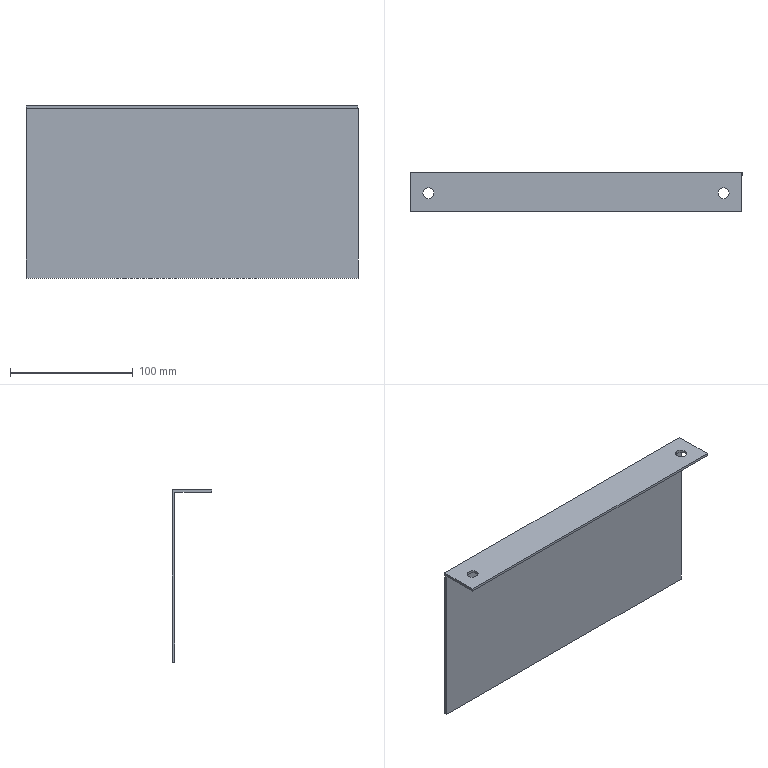Part | STEP file | lll_id2182_x_t | 1 solid | 10 faces | box 270 x 32 x 140 mm | volume 91546 mm3 | plane 8 | cylinder 2 | commonest cylinder face diameters 9 x2
STEP:
#1=CARTESIAN_POINT('',(554.935,-441.,2.5));
#2=VERTEX_POINT('',#1);
#3=CARTESIAN_POINT('',(554.935,-439.,2.5));
#4=VERTEX_POINT('',#3);
#5=CARTESIAN_POINT('',(554.935,-441.,2.5));
#6=DIRECTION('',(0.,1.,0.));
#7=VECTOR('',#6,1.);
#8=LINE('',#5,#7);
#9=EDGE_CURVE('',#2,#4,#8,.T.);
#10=ORIENTED_EDGE('',*,*,#9,.T.);
#11=CARTESIAN_POINT('',(824.935,-439.,2.5));
#12=VERTEX_POINT('',#11);
#13=CARTESIAN_POINT('',(499.935,-439.,2.5));
#14=DIRECTION('',(1.,0.,0.));
#15=VECTOR('',#14,1.);
#16=LINE('',#13,#15);
#17=EDGE_CURVE('',#4,#12,#16,.T.);
#18=ORIENTED_EDGE('',*,*,#17,.T.);
#19=CARTESIAN_POINT('',(824.935,-441.,2.5));
#20=VERTEX_POINT('',#19);
#21=CARTESIAN_POINT('',(824.935,45.,2.5));
#22=DIRECTION('',(0.,1.,0.));
#23=VECTOR('',#22,1.);
#24=LINE('',#21,#23);
#25=EDGE_CURVE('',#20,#12,#24,.T.);
#26=ORIENTED_EDGE('',*,*,#25,.F.);
#27=CARTESIAN_POINT('',(499.935,-441.,2.5));
#28=DIRECTION('',(1.,0.,0.));
#29=VECTOR('',#28,1.);
#30=LINE('',#27,#29);
#31=EDGE_CURVE('',#2,#20,#30,.T.);
#32=ORIENTED_EDGE('',*,*,#31,.F.);
#33=EDGE_LOOP('',(#10,#18,#26,#32));
#34=FACE_OUTER_BOUND('',#33,.T.);
#35=CARTESIAN_POINT('',(1692.435,45.,2.5));
#36=DIRECTION('',(0.,0.,-1.));
#37=DIRECTION('',(-1.,0.,0.));
#38=AXIS2_PLACEMENT_3D('',#35,#36,#37);
#39=PLANE('',#38);
#40=ADVANCED_FACE('',(#34),#39,.T.);
#41=CARTESIAN_POINT('',(824.935,-441.,140.5));
#42=VERTEX_POINT('',#41);
#43=CARTESIAN_POINT('',(554.935,-441.,140.5));
#44=VERTEX_POINT('',#43);
#45=CARTESIAN_POINT('',(499.935,-441.,140.5));
#46=DIRECTION('',(-1.,0.,0.));
#47=VECTOR('',#46,1.);
#48=LINE('',#45,#47);
#49=EDGE_CURVE('',#42,#44,#48,.T.);
#50=ORIENTED_EDGE('',*,*,#49,.T.);
#51=CARTESIAN_POINT('',(554.935,-441.,142.5));
#52=DIRECTION('',(0.,0.,-1.));
#53=VECTOR('',#52,1.);
#54=LINE('',#51,#53);
#55=EDGE_CURVE('',#44,#2,#54,.T.);
#56=ORIENTED_EDGE('',*,*,#55,.T.);
#57=ORIENTED_EDGE('',*,*,#31,.T.);
#58=CARTESIAN_POINT('',(824.935,-441.,-78.5));
#59=DIRECTION('',(0.,0.,1.));
#60=VECTOR('',#59,1.);
#61=LINE('',#58,#60);
#62=EDGE_CURVE('',#20,#42,#61,.T.);
#63=ORIENTED_EDGE('',*,*,#62,.T.);
#64=EDGE_LOOP('',(#50,#56,#57,#63));
#65=FACE_OUTER_BOUND('',#64,.T.);
#66=CARTESIAN_POINT('',(499.935,-441.,-78.5));
#67=DIRECTION('',(0.,1.,0.));
#68=DIRECTION('',(0.,0.,-1.));
#69=AXIS2_PLACEMENT_3D('',#66,#67,#68);
#70=PLANE('',#69);
#71=ADVANCED_FACE('',(#65),#70,.F.);
#72=CARTESIAN_POINT('',(554.935,-439.,142.5));
#73=VERTEX_POINT('',#72);
#74=CARTESIAN_POINT('',(554.935,-439.,-78.5));
#75=DIRECTION('',(0.,0.,-1.));
#76=VECTOR('',#75,1.);
#77=LINE('',#74,#76);
#78=EDGE_CURVE('',#73,#4,#77,.T.);
#79=ORIENTED_EDGE('',*,*,#78,.F.);
#80=CARTESIAN_POINT('',(824.935,-439.,142.5));
#81=VERTEX_POINT('',#80);
#82=CARTESIAN_POINT('',(499.935,-439.,142.5));
#83=DIRECTION('',(-1.,0.,0.));
#84=VECTOR('',#83,1.);
#85=LINE('',#82,#84);
#86=EDGE_CURVE('',#81,#73,#85,.T.);
#87=ORIENTED_EDGE('',*,*,#86,.F.);
#88=CARTESIAN_POINT('',(824.935,-439.,-78.5));
#89=DIRECTION('',(0.,0.,1.));
#90=VECTOR('',#89,1.);
#91=LINE('',#88,#90);
#92=EDGE_CURVE('',#12,#81,#91,.T.);
#93=ORIENTED_EDGE('',*,*,#92,.F.);
#94=ORIENTED_EDGE('',*,*,#17,.F.);
#95=EDGE_LOOP('',(#79,#87,#93,#94));
#96=FACE_OUTER_BOUND('',#95,.T.);
#97=CARTESIAN_POINT('',(499.935,-439.,-78.5));
#98=DIRECTION('',(0.,1.,0.));
#99=DIRECTION('',(0.,0.,-1.));
#100=AXIS2_PLACEMENT_3D('',#97,#98,#99);
#101=PLANE('',#100);
#102=ADVANCED_FACE('',(#96),#101,.T.);
#103=ORIENTED_EDGE('',*,*,#9,.F.);
#104=ORIENTED_EDGE('',*,*,#55,.F.);
#105=CARTESIAN_POINT('',(554.935,-471.,140.5));
#106=VERTEX_POINT('',#105);
#107=CARTESIAN_POINT('',(554.935,-441.,140.5));
#108=DIRECTION('',(0.,1.,0.));
#109=VECTOR('',#108,1.);
#110=LINE('',#107,#109);
#111=EDGE_CURVE('',#106,#44,#110,.T.);
#112=ORIENTED_EDGE('',*,*,#111,.F.);
#113=CARTESIAN_POINT('',(554.935,-471.,142.5));
#114=VERTEX_POINT('',#113);
#115=CARTESIAN_POINT('',(554.935,-471.,142.5));
#116=DIRECTION('',(0.,0.,-1.));
#117=VECTOR('',#116,1.);
#118=LINE('',#115,#117);
#119=EDGE_CURVE('',#114,#106,#118,.T.);
#120=ORIENTED_EDGE('',*,*,#119,.F.);
#121=CARTESIAN_POINT('',(554.935,-441.,142.5));
#122=DIRECTION('',(0.,1.,0.));
#123=VECTOR('',#122,1.);
#124=LINE('',#121,#123);
#125=EDGE_CURVE('',#114,#73,#124,.T.);
#126=ORIENTED_EDGE('',*,*,#125,.T.);
#127=ORIENTED_EDGE('',*,*,#78,.T.);
#128=EDGE_LOOP('',(#103,#104,#112,#120,#126,#127));
#129=FACE_OUTER_BOUND('',#128,.T.);
#130=CARTESIAN_POINT('',(554.935,-441.,142.5));
#131=DIRECTION('',(-1.,0.,0.));
#132=DIRECTION('',(0.,0.,-1.));
#133=AXIS2_PLACEMENT_3D('',#130,#131,#132);
#134=PLANE('',#133);
#135=ADVANCED_FACE('',(#129),#134,.T.);
#136=ORIENTED_EDGE('',*,*,#119,.T.);
#137=CARTESIAN_POINT('',(824.935,-471.,140.5));
#138=VERTEX_POINT('',#137);
#139=CARTESIAN_POINT('',(499.935,-471.,140.5));
#140=DIRECTION('',(-1.,0.,0.));
#141=VECTOR('',#140,1.);
#142=LINE('',#139,#141);
#143=EDGE_CURVE('',#138,#106,#142,.T.);
#144=ORIENTED_EDGE('',*,*,#143,.F.);
#145=CARTESIAN_POINT('',(824.935,-471.,142.5));
#146=VERTEX_POINT('',#145);
#147=CARTESIAN_POINT('',(824.935,-471.,142.5));
#148=DIRECTION('',(0.,0.,-1.));
#149=VECTOR('',#148,1.);
#150=LINE('',#147,#149);
#151=EDGE_CURVE('',#146,#138,#150,.T.);
#152=ORIENTED_EDGE('',*,*,#151,.F.);
#153=CARTESIAN_POINT('',(499.935,-471.,142.5));
#154=DIRECTION('',(-1.,0.,0.));
#155=VECTOR('',#154,1.);
#156=LINE('',#153,#155);
#157=EDGE_CURVE('',#146,#114,#156,.T.);
#158=ORIENTED_EDGE('',*,*,#157,.T.);
#159=EDGE_LOOP('',(#136,#144,#152,#158));
#160=FACE_OUTER_BOUND('',#159,.T.);
#161=CARTESIAN_POINT('',(499.935,-471.,142.5));
#162=DIRECTION('',(0.,-1.,0.));
#163=DIRECTION('',(1.,0.,0.));
#164=AXIS2_PLACEMENT_3D('',#161,#162,#163);
#165=PLANE('',#164);
#166=ADVANCED_FACE('',(#160),#165,.T.);
#167=CARTESIAN_POINT('',(824.935,-441.,142.5));
#168=DIRECTION('',(0.,1.,0.));
#169=VECTOR('',#168,1.);
#170=LINE('',#167,#169);
#171=EDGE_CURVE('',#146,#81,#170,.T.);
#172=ORIENTED_EDGE('',*,*,#171,.F.);
#173=ORIENTED_EDGE('',*,*,#151,.T.);
#174=CARTESIAN_POINT('',(824.935,-441.,140.5));
#175=DIRECTION('',(0.,1.,0.));
#176=VECTOR('',#175,1.);
#177=LINE('',#174,#176);
#178=EDGE_CURVE('',#138,#42,#177,.T.);
#179=ORIENTED_EDGE('',*,*,#178,.T.);
#180=ORIENTED_EDGE('',*,*,#62,.F.);
#181=ORIENTED_EDGE('',*,*,#25,.T.);
#182=ORIENTED_EDGE('',*,*,#92,.T.);
#183=EDGE_LOOP('',(#172,#173,#179,#180,#181,#182));
#184=FACE_OUTER_BOUND('',#183,.T.);
#185=CARTESIAN_POINT('',(824.935,-441.,-78.5));
#186=DIRECTION('',(-1.,0.,0.));
#187=DIRECTION('',(0.,0.,-1.));
#188=AXIS2_PLACEMENT_3D('',#185,#186,#187);
#189=PLANE('',#188);
#190=ADVANCED_FACE('',(#184),#189,.F.);
#191=CARTESIAN_POINT('',(805.435,-456.,142.5));
#192=VERTEX_POINT('',#191);
#193=CARTESIAN_POINT('',(809.935,-456.,142.5));
#194=DIRECTION('',(0.,0.,-1.));
#195=DIRECTION('',(-1.,0.,0.));
#196=AXIS2_PLACEMENT_3D('',#193,#194,#195);
#197=CIRCLE('',#196,4.5);
#198=EDGE_CURVE('',#192,#192,#197,.T.);
#199=ORIENTED_EDGE('',*,*,#198,.F.);
#200=EDGE_LOOP('',(#199));
#201=FACE_BOUND('',#200,.T.);
#202=CARTESIAN_POINT('',(814.435,-456.,140.5));
#203=VERTEX_POINT('',#202);
#204=CARTESIAN_POINT('',(809.935,-456.,140.5));
#205=DIRECTION('',(0.,0.,-1.));
#206=DIRECTION('',(1.,0.,0.));
#207=AXIS2_PLACEMENT_3D('',#204,#205,#206);
#208=CIRCLE('',#207,4.5);
#209=EDGE_CURVE('',#203,#203,#208,.T.);
#210=ORIENTED_EDGE('',*,*,#209,.T.);
#211=EDGE_LOOP('',(#210));
#212=FACE_BOUND('',#211,.T.);
#213=CARTESIAN_POINT('',(809.935,-456.,140.5));
#214=DIRECTION('',(0.,0.,1.));
#215=DIRECTION('',(1.,0.,0.));
#216=AXIS2_PLACEMENT_3D('',#213,#214,#215);
#217=CYLINDRICAL_SURFACE('',#216,4.5);
#218=ADVANCED_FACE('',(#201,#212),#217,.F.);
#219=CARTESIAN_POINT('',(565.435,-456.,142.5));
#220=VERTEX_POINT('',#219);
#221=CARTESIAN_POINT('',(569.935,-456.,142.5));
#222=DIRECTION('',(0.,0.,-1.));
#223=DIRECTION('',(-1.,0.,0.));
#224=AXIS2_PLACEMENT_3D('',#221,#222,#223);
#225=CIRCLE('',#224,4.5);
#226=EDGE_CURVE('',#220,#220,#225,.T.);
#227=ORIENTED_EDGE('',*,*,#226,.F.);
#228=EDGE_LOOP('',(#227));
#229=FACE_BOUND('',#228,.T.);
#230=CARTESIAN_POINT('',(565.435,-456.,140.5));
#231=VERTEX_POINT('',#230);
#232=CARTESIAN_POINT('',(569.935,-456.,140.5));
#233=DIRECTION('',(0.,0.,-1.));
#234=DIRECTION('',(-1.,0.,0.));
#235=AXIS2_PLACEMENT_3D('',#232,#233,#234);
#236=CIRCLE('',#235,4.5);
#237=EDGE_CURVE('',#231,#231,#236,.T.);
#238=ORIENTED_EDGE('',*,*,#237,.T.);
#239=EDGE_LOOP('',(#238));
#240=FACE_BOUND('',#239,.T.);
#241=CARTESIAN_POINT('',(569.935,-456.,140.5));
#242=DIRECTION('',(0.,0.,1.));
#243=DIRECTION('',(-1.,0.,0.));
#244=AXIS2_PLACEMENT_3D('',#241,#242,#243);
#245=CYLINDRICAL_SURFACE('',#244,4.5);
#246=ADVANCED_FACE('',(#229,#240),#245,.F.);
#247=ORIENTED_EDGE('',*,*,#226,.T.);
#248=EDGE_LOOP('',(#247));
#249=FACE_BOUND('',#248,.T.);
#250=ORIENTED_EDGE('',*,*,#198,.T.);
#251=EDGE_LOOP('',(#250));
#252=FACE_BOUND('',#251,.T.);
#253=ORIENTED_EDGE('',*,*,#171,.T.);
#254=ORIENTED_EDGE('',*,*,#86,.T.);
#255=ORIENTED_EDGE('',*,*,#125,.F.);
#256=ORIENTED_EDGE('',*,*,#157,.F.);
#257=EDGE_LOOP('',(#253,#254,#255,#256));
#258=FACE_BOUND('',#257,.T.);
#259=CARTESIAN_POINT('',(499.935,-441.,142.5));
#260=DIRECTION('',(0.,0.,-1.));
#261=DIRECTION('',(1.,0.,0.));
#262=AXIS2_PLACEMENT_3D('',#259,#260,#261);
#263=PLANE('',#262);
#264=ADVANCED_FACE('',(#249,#252,#258),#263,.F.);
#265=ORIENTED_EDGE('',*,*,#237,.F.);
#266=EDGE_LOOP('',(#265));
#267=FACE_BOUND('',#266,.T.);
#268=ORIENTED_EDGE('',*,*,#209,.F.);
#269=EDGE_LOOP('',(#268));
#270=FACE_BOUND('',#269,.T.);
#271=ORIENTED_EDGE('',*,*,#178,.F.);
#272=ORIENTED_EDGE('',*,*,#143,.T.);
#273=ORIENTED_EDGE('',*,*,#111,.T.);
#274=ORIENTED_EDGE('',*,*,#49,.F.);
#275=EDGE_LOOP('',(#271,#272,#273,#274));
#276=FACE_BOUND('',#275,.T.);
#277=CARTESIAN_POINT('',(499.935,-441.,140.5));
#278=DIRECTION('',(0.,0.,-1.));
#279=DIRECTION('',(1.,0.,0.));
#280=AXIS2_PLACEMENT_3D('',#277,#278,#279);
#281=PLANE('',#280);
#282=ADVANCED_FACE('',(#267,#270,#276),#281,.T.);
#283=CLOSED_SHELL('',(#40,#71,#102,#135,#166,#190,#218,#246,#264,#282));
#284=MANIFOLD_SOLID_BREP('',#283);
#285=(LENGTH_UNIT()NAMED_UNIT(*)SI_UNIT(.MILLI.,.METRE.));
#286=UNCERTAINTY_MEASURE_WITH_UNIT(LENGTH_MEASURE(0.00002),#285,'','');
#287=(NAMED_UNIT(*)PLANE_ANGLE_UNIT()SI_UNIT($,.RADIAN.));
#288=PLANE_ANGLE_MEASURE_WITH_UNIT(PLANE_ANGLE_MEASURE(0.01745),#287);
#289=DIMENSIONAL_EXPONENTS(0.,0.,0.,0.,0.,0.,0.);
#290=(CONVERSION_BASED_UNIT('DEGREE',#288)NAMED_UNIT(#289)PLANE_ANGLE_UNIT());
#291=(NAMED_UNIT(*)SI_UNIT($,.STERADIAN.)SOLID_ANGLE_UNIT());
#292=(GEOMETRIC_REPRESENTATION_CONTEXT(3)GLOBAL_UNCERTAINTY_ASSIGNED_CONTEXT((#286))GLOBAL_UNIT_ASSIGNED_CONTEXT((#285,#290,#291))REPRESENTATION_CONTEXT('',''));
#293=ADVANCED_BREP_SHAPE_REPRESENTATION('',(#284),#292);